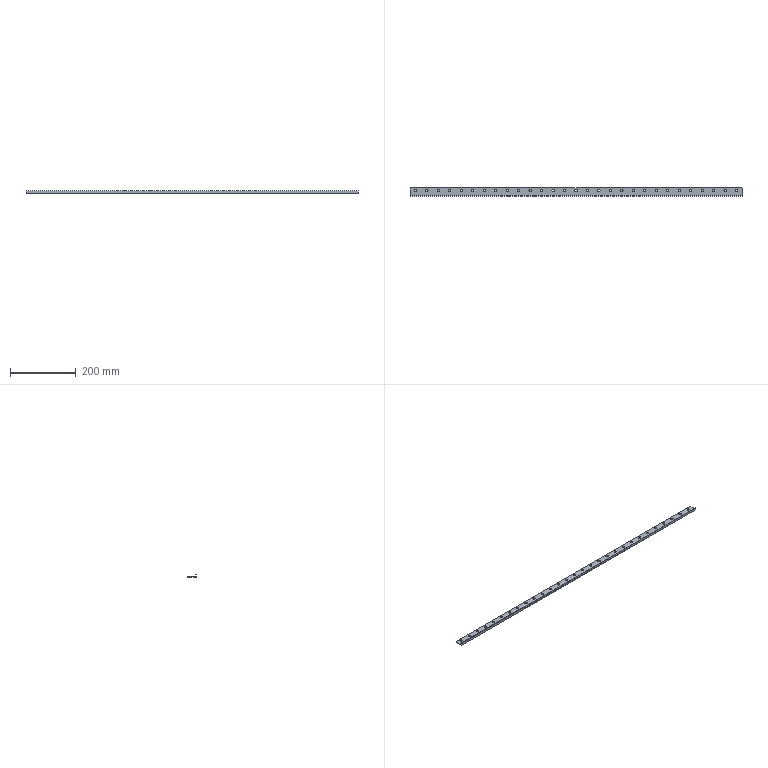Part | STEP file | PLATE_0829_041_CRONWB29 | 1 solid | 68 faces | box 1013 x 25 x 7 mm | volume 47472 mm3 | cylinder 58 | plane 10 | commonest cylinder face diameters 7 x58